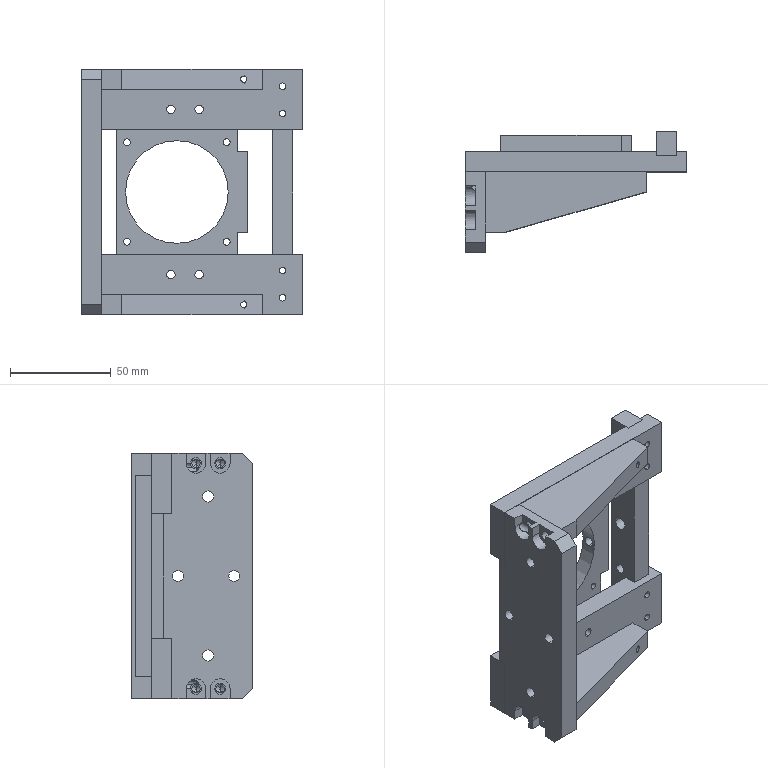Part | NX | features BREP 6 | 7 solids | 260 faces | box 110 x 60 x 122 mm | volume 184982 mm3 | cylinder 140 | plane 90 | cone 30 | commonest cylinder face diameters 4.2 x44 5.5 x40 3.3 x16 9.8 x14 4.5 x8 8 x8